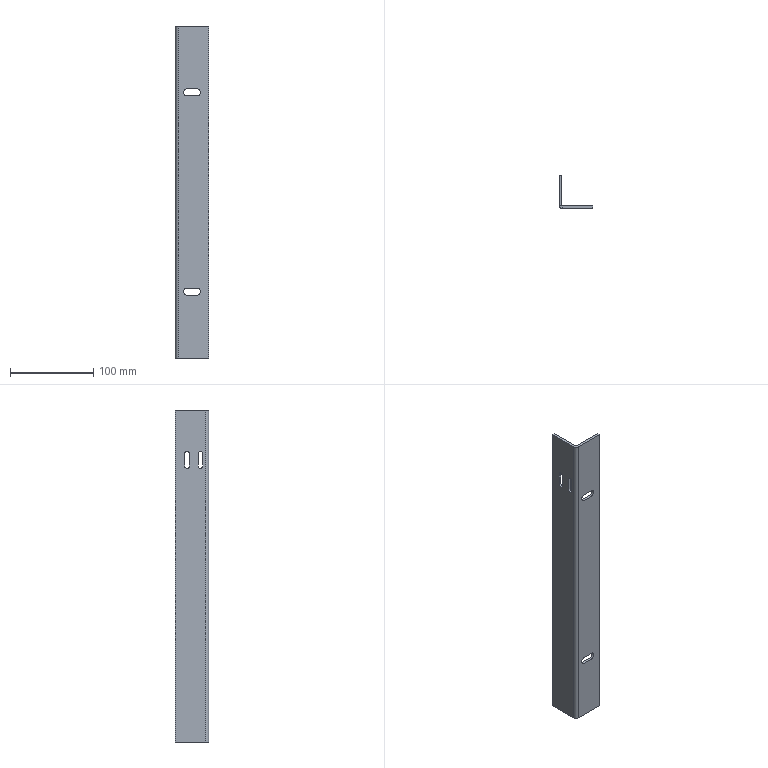Part | STEP file | PN_0031 (stop side plate) | 1 solid | 32 faces | box 40 x 40 x 400 mm | volume 89658 mm3 | plane 20 | cylinder 12 | commonest cylinder face diameters 5.5 x6 8.5 x4 1.473 x1 7.473 x1